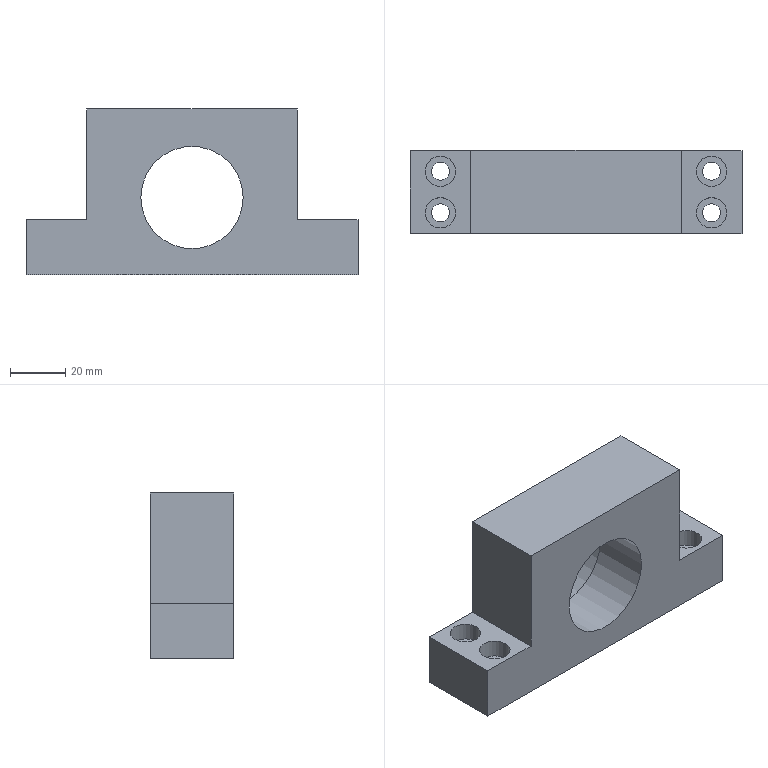Part | NX | features CBORE_HOLE 4, DATUM_CSYS 4, SKETCH 3, EXTRUDE 2, HOLE PACKAGE 1 | 1 solid | 25 faces | box 120 x 30 x 60 mm | volume 123889 mm3 | plane 15 | cylinder 10 | commonest cylinder face diameters 6.5 x4 11 x4 37 x1 42 x1
STEP:
#1=CARTESIAN_POINT('',(21.,15.,28.));
#2=VERTEX_POINT('',#1);
#3=CARTESIAN_POINT('',(0.,15.,28.));
#4=DIRECTION('',(0.,-1.,0.));
#5=DIRECTION('',(1.,0.,0.));
#6=AXIS2_PLACEMENT_3D('',#3,#4,#5);
#7=CIRCLE('',#6,21.);
#8=EDGE_CURVE('',#2,#2,#7,.T.);
#9=ORIENTED_EDGE('',*,*,#8,.F.);
#10=EDGE_LOOP('',(#9));
#11=FACE_BOUND('',#10,.T.);
#12=CARTESIAN_POINT('',(21.,6.,28.));
#13=VERTEX_POINT('',#12);
#14=CARTESIAN_POINT('',(0.,6.,28.));
#15=DIRECTION('',(0.,-1.,0.));
#16=DIRECTION('',(1.,0.,0.));
#17=AXIS2_PLACEMENT_3D('',#14,#15,#16);
#18=CIRCLE('',#17,21.);
#19=EDGE_CURVE('',#13,#13,#18,.T.);
#20=ORIENTED_EDGE('',*,*,#19,.T.);
#21=EDGE_LOOP('',(#20));
#22=FACE_BOUND('',#21,.T.);
#23=CARTESIAN_POINT('',(0.,-15.,28.));
#24=DIRECTION('',(0.,1.,0.));
#25=DIRECTION('',(0.,0.,1.));
#26=AXIS2_PLACEMENT_3D('',#23,#24,#25);
#27=CYLINDRICAL_SURFACE('',#26,21.);
#28=ADVANCED_FACE('',(#11,#22),#27,.F.);
#29=CARTESIAN_POINT('',(-60.,15.,20.));
#30=VERTEX_POINT('',#29);
#31=CARTESIAN_POINT('',(-60.,15.,0.));
#32=VERTEX_POINT('',#31);
#33=CARTESIAN_POINT('',(-60.,15.,20.));
#34=DIRECTION('',(0.,0.,-1.));
#35=VECTOR('',#34,1000.);
#36=LINE('',#33,#35);
#37=EDGE_CURVE('',#30,#32,#36,.T.);
#38=ORIENTED_EDGE('',*,*,#37,.T.);
#39=CARTESIAN_POINT('',(-60.,-15.,0.));
#40=VERTEX_POINT('',#39);
#41=CARTESIAN_POINT('',(-60.,-15.,0.));
#42=DIRECTION('',(0.,1.,0.));
#43=VECTOR('',#42,1000.);
#44=LINE('',#41,#43);
#45=EDGE_CURVE('',#40,#32,#44,.T.);
#46=ORIENTED_EDGE('',*,*,#45,.F.);
#47=CARTESIAN_POINT('',(-60.,-15.,20.));
#48=VERTEX_POINT('',#47);
#49=CARTESIAN_POINT('',(-60.,-15.,20.));
#50=DIRECTION('',(0.,0.,-1.));
#51=VECTOR('',#50,1000.);
#52=LINE('',#49,#51);
#53=EDGE_CURVE('',#48,#40,#52,.T.);
#54=ORIENTED_EDGE('',*,*,#53,.F.);
#55=CARTESIAN_POINT('',(-60.,-15.,20.));
#56=DIRECTION('',(0.,1.,0.));
#57=VECTOR('',#56,1000.);
#58=LINE('',#55,#57);
#59=EDGE_CURVE('',#48,#30,#58,.T.);
#60=ORIENTED_EDGE('',*,*,#59,.T.);
#61=EDGE_LOOP('',(#38,#46,#54,#60));
#62=FACE_BOUND('',#61,.T.);
#63=CARTESIAN_POINT('',(-60.,-15.,20.));
#64=DIRECTION('',(1.,0.,0.));
#65=DIRECTION('',(0.,0.,-1.));
#66=AXIS2_PLACEMENT_3D('',#63,#64,#65);
#67=PLANE('',#66);
#68=ADVANCED_FACE('',(#62),#67,.F.);
#69=CARTESIAN_POINT('',(52.25,7.5,0.));
#70=VERTEX_POINT('',#69);
#71=CARTESIAN_POINT('',(49.,7.5,0.));
#72=DIRECTION('',(0.,0.,1.));
#73=DIRECTION('',(1.,0.,0.));
#74=AXIS2_PLACEMENT_3D('',#71,#72,#73);
#75=CIRCLE('',#74,3.25);
#76=EDGE_CURVE('',#70,#70,#75,.T.);
#77=ORIENTED_EDGE('',*,*,#76,.T.);
#78=EDGE_LOOP('',(#77));
#79=FACE_BOUND('',#78,.T.);
#80=CARTESIAN_POINT('',(52.25,-7.5,0.));
#81=VERTEX_POINT('',#80);
#82=CARTESIAN_POINT('',(49.,-7.5,0.));
#83=DIRECTION('',(0.,0.,1.));
#84=DIRECTION('',(1.,0.,0.));
#85=AXIS2_PLACEMENT_3D('',#82,#83,#84);
#86=CIRCLE('',#85,3.25);
#87=EDGE_CURVE('',#81,#81,#86,.T.);
#88=ORIENTED_EDGE('',*,*,#87,.T.);
#89=EDGE_LOOP('',(#88));
#90=FACE_BOUND('',#89,.T.);
#91=CARTESIAN_POINT('',(-45.75,-7.5,0.));
#92=VERTEX_POINT('',#91);
#93=CARTESIAN_POINT('',(-49.,-7.5,0.));
#94=DIRECTION('',(0.,0.,1.));
#95=DIRECTION('',(1.,0.,0.));
#96=AXIS2_PLACEMENT_3D('',#93,#94,#95);
#97=CIRCLE('',#96,3.25);
#98=EDGE_CURVE('',#92,#92,#97,.T.);
#99=ORIENTED_EDGE('',*,*,#98,.T.);
#100=EDGE_LOOP('',(#99));
#101=FACE_BOUND('',#100,.T.);
#102=CARTESIAN_POINT('',(-45.75,7.5,0.));
#103=VERTEX_POINT('',#102);
#104=CARTESIAN_POINT('',(-49.,7.5,0.));
#105=DIRECTION('',(0.,0.,1.));
#106=DIRECTION('',(1.,0.,0.));
#107=AXIS2_PLACEMENT_3D('',#104,#105,#106);
#108=CIRCLE('',#107,3.25);
#109=EDGE_CURVE('',#103,#103,#108,.T.);
#110=ORIENTED_EDGE('',*,*,#109,.T.);
#111=EDGE_LOOP('',(#110));
#112=FACE_BOUND('',#111,.T.);
#113=CARTESIAN_POINT('',(60.,15.,0.));
#114=VERTEX_POINT('',#113);
#115=CARTESIAN_POINT('',(-60.,15.,0.));
#116=DIRECTION('',(1.,0.,0.));
#117=VECTOR('',#116,1000.);
#118=LINE('',#115,#117);
#119=EDGE_CURVE('',#32,#114,#118,.T.);
#120=ORIENTED_EDGE('',*,*,#119,.T.);
#121=CARTESIAN_POINT('',(60.,-15.,0.));
#122=VERTEX_POINT('',#121);
#123=CARTESIAN_POINT('',(60.,-15.,0.));
#124=DIRECTION('',(0.,1.,0.));
#125=VECTOR('',#124,1000.);
#126=LINE('',#123,#125);
#127=EDGE_CURVE('',#122,#114,#126,.T.);
#128=ORIENTED_EDGE('',*,*,#127,.F.);
#129=CARTESIAN_POINT('',(-60.,-15.,0.));
#130=DIRECTION('',(1.,0.,0.));
#131=VECTOR('',#130,1000.);
#132=LINE('',#129,#131);
#133=EDGE_CURVE('',#40,#122,#132,.T.);
#134=ORIENTED_EDGE('',*,*,#133,.F.);
#135=ORIENTED_EDGE('',*,*,#45,.T.);
#136=EDGE_LOOP('',(#120,#128,#134,#135));
#137=FACE_BOUND('',#136,.T.);
#138=CARTESIAN_POINT('',(-60.,-15.,0.));
#139=DIRECTION('',(0.,0.,1.));
#140=DIRECTION('',(1.,0.,0.));
#141=AXIS2_PLACEMENT_3D('',#138,#139,#140);
#142=PLANE('',#141);
#143=ADVANCED_FACE('',(#79,#90,#101,#112,#137),#142,.F.);
#144=CARTESIAN_POINT('',(60.,15.,20.));
#145=VERTEX_POINT('',#144);
#146=CARTESIAN_POINT('',(60.,15.,0.));
#147=DIRECTION('',(0.,0.,1.));
#148=VECTOR('',#147,1000.);
#149=LINE('',#146,#148);
#150=EDGE_CURVE('',#114,#145,#149,.T.);
#151=ORIENTED_EDGE('',*,*,#150,.T.);
#152=CARTESIAN_POINT('',(60.,-15.,20.));
#153=VERTEX_POINT('',#152);
#154=CARTESIAN_POINT('',(60.,-15.,20.));
#155=DIRECTION('',(0.,1.,0.));
#156=VECTOR('',#155,1000.);
#157=LINE('',#154,#156);
#158=EDGE_CURVE('',#153,#145,#157,.T.);
#159=ORIENTED_EDGE('',*,*,#158,.F.);
#160=CARTESIAN_POINT('',(60.,-15.,0.));
#161=DIRECTION('',(0.,0.,1.));
#162=VECTOR('',#161,1000.);
#163=LINE('',#160,#162);
#164=EDGE_CURVE('',#122,#153,#163,.T.);
#165=ORIENTED_EDGE('',*,*,#164,.F.);
#166=ORIENTED_EDGE('',*,*,#127,.T.);
#167=EDGE_LOOP('',(#151,#159,#165,#166));
#168=FACE_BOUND('',#167,.T.);
#169=CARTESIAN_POINT('',(60.,-15.,0.));
#170=DIRECTION('',(-1.,0.,0.));
#171=DIRECTION('',(0.,0.,1.));
#172=AXIS2_PLACEMENT_3D('',#169,#170,#171);
#173=PLANE('',#172);
#174=ADVANCED_FACE('',(#168),#173,.F.);
#175=CARTESIAN_POINT('',(43.5,7.5,20.));
#176=VERTEX_POINT('',#175);
#177=CARTESIAN_POINT('',(49.,7.5,20.));
#178=DIRECTION('',(0.,0.,-1.));
#179=DIRECTION('',(-1.,0.,0.));
#180=AXIS2_PLACEMENT_3D('',#177,#178,#179);
#181=CIRCLE('',#180,5.5);
#182=EDGE_CURVE('',#176,#176,#181,.T.);
#183=ORIENTED_EDGE('',*,*,#182,.T.);
#184=EDGE_LOOP('',(#183));
#185=FACE_BOUND('',#184,.T.);
#186=CARTESIAN_POINT('',(43.5,-7.5,20.));
#187=VERTEX_POINT('',#186);
#188=CARTESIAN_POINT('',(49.,-7.5,20.));
#189=DIRECTION('',(0.,0.,-1.));
#190=DIRECTION('',(-1.,0.,0.));
#191=AXIS2_PLACEMENT_3D('',#188,#189,#190);
#192=CIRCLE('',#191,5.5);
#193=EDGE_CURVE('',#187,#187,#192,.T.);
#194=ORIENTED_EDGE('',*,*,#193,.T.);
#195=EDGE_LOOP('',(#194));
#196=FACE_BOUND('',#195,.T.);
#197=CARTESIAN_POINT('',(38.,15.,20.));
#198=VERTEX_POINT('',#197);
#199=CARTESIAN_POINT('',(60.,15.,20.));
#200=DIRECTION('',(-1.,0.,0.));
#201=VECTOR('',#200,1000.);
#202=LINE('',#199,#201);
#203=EDGE_CURVE('',#145,#198,#202,.T.);
#204=ORIENTED_EDGE('',*,*,#203,.T.);
#205=CARTESIAN_POINT('',(38.,-15.,20.));
#206=VERTEX_POINT('',#205);
#207=CARTESIAN_POINT('',(38.,-15.,20.));
#208=DIRECTION('',(0.,1.,0.));
#209=VECTOR('',#208,1000.);
#210=LINE('',#207,#209);
#211=EDGE_CURVE('',#206,#198,#210,.T.);
#212=ORIENTED_EDGE('',*,*,#211,.F.);
#213=CARTESIAN_POINT('',(60.,-15.,20.));
#214=DIRECTION('',(-1.,0.,0.));
#215=VECTOR('',#214,1000.);
#216=LINE('',#213,#215);
#217=EDGE_CURVE('',#153,#206,#216,.T.);
#218=ORIENTED_EDGE('',*,*,#217,.F.);
#219=ORIENTED_EDGE('',*,*,#158,.T.);
#220=EDGE_LOOP('',(#204,#212,#218,#219));
#221=FACE_BOUND('',#220,.T.);
#222=CARTESIAN_POINT('',(60.,-15.,20.));
#223=DIRECTION('',(0.,0.,-1.));
#224=DIRECTION('',(-1.,0.,0.));
#225=AXIS2_PLACEMENT_3D('',#222,#223,#224);
#226=PLANE('',#225);
#227=ADVANCED_FACE('',(#185,#196,#221),#226,.F.);
#228=CARTESIAN_POINT('',(38.,15.,60.));
#229=VERTEX_POINT('',#228);
#230=CARTESIAN_POINT('',(38.,15.,20.));
#231=DIRECTION('',(0.,0.,1.));
#232=VECTOR('',#231,1000.);
#233=LINE('',#230,#232);
#234=EDGE_CURVE('',#198,#229,#233,.T.);
#235=ORIENTED_EDGE('',*,*,#234,.T.);
#236=CARTESIAN_POINT('',(38.,-15.,60.));
#237=VERTEX_POINT('',#236);
#238=CARTESIAN_POINT('',(38.,-15.,60.));
#239=DIRECTION('',(0.,1.,0.));
#240=VECTOR('',#239,1000.);
#241=LINE('',#238,#240);
#242=EDGE_CURVE('',#237,#229,#241,.T.);
#243=ORIENTED_EDGE('',*,*,#242,.F.);
#244=CARTESIAN_POINT('',(38.,-15.,20.));
#245=DIRECTION('',(0.,0.,1.));
#246=VECTOR('',#245,1000.);
#247=LINE('',#244,#246);
#248=EDGE_CURVE('',#206,#237,#247,.T.);
#249=ORIENTED_EDGE('',*,*,#248,.F.);
#250=ORIENTED_EDGE('',*,*,#211,.T.);
#251=EDGE_LOOP('',(#235,#243,#249,#250));
#252=FACE_BOUND('',#251,.T.);
#253=CARTESIAN_POINT('',(38.,-15.,20.));
#254=DIRECTION('',(-1.,0.,0.));
#255=DIRECTION('',(0.,0.,1.));
#256=AXIS2_PLACEMENT_3D('',#253,#254,#255);
#257=PLANE('',#256);
#258=ADVANCED_FACE('',(#252),#257,.F.);
#259=CARTESIAN_POINT('',(-38.,15.,60.));
#260=VERTEX_POINT('',#259);
#261=CARTESIAN_POINT('',(38.,15.,60.));
#262=DIRECTION('',(-1.,0.,0.));
#263=VECTOR('',#262,1000.);
#264=LINE('',#261,#263);
#265=EDGE_CURVE('',#229,#260,#264,.T.);
#266=ORIENTED_EDGE('',*,*,#265,.T.);
#267=CARTESIAN_POINT('',(-38.,-15.,60.));
#268=VERTEX_POINT('',#267);
#269=CARTESIAN_POINT('',(-38.,-15.,60.));
#270=DIRECTION('',(0.,1.,0.));
#271=VECTOR('',#270,1000.);
#272=LINE('',#269,#271);
#273=EDGE_CURVE('',#268,#260,#272,.T.);
#274=ORIENTED_EDGE('',*,*,#273,.F.);
#275=CARTESIAN_POINT('',(38.,-15.,60.));
#276=DIRECTION('',(-1.,0.,0.));
#277=VECTOR('',#276,1000.);
#278=LINE('',#275,#277);
#279=EDGE_CURVE('',#237,#268,#278,.T.);
#280=ORIENTED_EDGE('',*,*,#279,.F.);
#281=ORIENTED_EDGE('',*,*,#242,.T.);
#282=EDGE_LOOP('',(#266,#274,#280,#281));
#283=FACE_BOUND('',#282,.T.);
#284=CARTESIAN_POINT('',(38.,-15.,60.));
#285=DIRECTION('',(0.,0.,-1.));
#286=DIRECTION('',(-1.,0.,0.));
#287=AXIS2_PLACEMENT_3D('',#284,#285,#286);
#288=PLANE('',#287);
#289=ADVANCED_FACE('',(#283),#288,.F.);
#290=CARTESIAN_POINT('',(-38.,15.,20.));
#291=VERTEX_POINT('',#290);
#292=CARTESIAN_POINT('',(-38.,15.,60.));
#293=DIRECTION('',(0.,0.,-1.));
#294=VECTOR('',#293,1000.);
#295=LINE('',#292,#294);
#296=EDGE_CURVE('',#260,#291,#295,.T.);
#297=ORIENTED_EDGE('',*,*,#296,.T.);
#298=CARTESIAN_POINT('',(-38.,-15.,20.));
#299=VERTEX_POINT('',#298);
#300=CARTESIAN_POINT('',(-38.,-15.,20.));
#301=DIRECTION('',(0.,1.,0.));
#302=VECTOR('',#301,1000.);
#303=LINE('',#300,#302);
#304=EDGE_CURVE('',#299,#291,#303,.T.);
#305=ORIENTED_EDGE('',*,*,#304,.F.);
#306=CARTESIAN_POINT('',(-38.,-15.,60.));
#307=DIRECTION('',(0.,0.,-1.));
#308=VECTOR('',#307,1000.);
#309=LINE('',#306,#308);
#310=EDGE_CURVE('',#268,#299,#309,.T.);
#311=ORIENTED_EDGE('',*,*,#310,.F.);
#312=ORIENTED_EDGE('',*,*,#273,.T.);
#313=EDGE_LOOP('',(#297,#305,#311,#312));
#314=FACE_BOUND('',#313,.T.);
#315=CARTESIAN_POINT('',(-38.,-15.,60.));
#316=DIRECTION('',(1.,0.,0.));
#317=DIRECTION('',(0.,0.,-1.));
#318=AXIS2_PLACEMENT_3D('',#315,#316,#317);
#319=PLANE('',#318);
#320=ADVANCED_FACE('',(#314),#319,.F.);
#321=CARTESIAN_POINT('',(-54.5,-7.5,20.));
#322=VERTEX_POINT('',#321);
#323=CARTESIAN_POINT('',(-49.,-7.5,20.));
#324=DIRECTION('',(0.,0.,-1.));
#325=DIRECTION('',(-1.,0.,0.));
#326=AXIS2_PLACEMENT_3D('',#323,#324,#325);
#327=CIRCLE('',#326,5.5);
#328=EDGE_CURVE('',#322,#322,#327,.T.);
#329=ORIENTED_EDGE('',*,*,#328,.T.);
#330=EDGE_LOOP('',(#329));
#331=FACE_BOUND('',#330,.T.);
#332=CARTESIAN_POINT('',(-54.5,7.5,20.));
#333=VERTEX_POINT('',#332);
#334=CARTESIAN_POINT('',(-49.,7.5,20.));
#335=DIRECTION('',(0.,0.,-1.));
#336=DIRECTION('',(-1.,0.,0.));
#337=AXIS2_PLACEMENT_3D('',#334,#335,#336);
#338=CIRCLE('',#337,5.5);
#339=EDGE_CURVE('',#333,#333,#338,.T.);
#340=ORIENTED_EDGE('',*,*,#339,.T.);
#341=EDGE_LOOP('',(#340));
#342=FACE_BOUND('',#341,.T.);
#343=CARTESIAN_POINT('',(-38.,15.,20.));
#344=DIRECTION('',(-1.,0.,0.));
#345=VECTOR('',#344,1000.);
#346=LINE('',#343,#345);
#347=EDGE_CURVE('',#291,#30,#346,.T.);
#348=ORIENTED_EDGE('',*,*,#347,.T.);
#349=ORIENTED_EDGE('',*,*,#59,.F.);
#350=CARTESIAN_POINT('',(-38.,-15.,20.));
#351=DIRECTION('',(-1.,0.,0.));
#352=VECTOR('',#351,1000.);
#353=LINE('',#350,#352);
#354=EDGE_CURVE('',#299,#48,#353,.T.);
#355=ORIENTED_EDGE('',*,*,#354,.F.);
#356=ORIENTED_EDGE('',*,*,#304,.T.);
#357=EDGE_LOOP('',(#348,#349,#355,#356));
#358=FACE_BOUND('',#357,.T.);
#359=CARTESIAN_POINT('',(-38.,-15.,20.));
#360=DIRECTION('',(0.,0.,-1.));
#361=DIRECTION('',(-1.,0.,0.));
#362=AXIS2_PLACEMENT_3D('',#359,#360,#361);
#363=PLANE('',#362);
#364=ADVANCED_FACE('',(#331,#342,#358),#363,.F.);
#365=ORIENTED_EDGE('',*,*,#53,.T.);
#366=ORIENTED_EDGE('',*,*,#133,.T.);
#367=ORIENTED_EDGE('',*,*,#164,.T.);
#368=ORIENTED_EDGE('',*,*,#217,.T.);
#369=ORIENTED_EDGE('',*,*,#248,.T.);
#370=ORIENTED_EDGE('',*,*,#279,.T.);
#371=ORIENTED_EDGE('',*,*,#310,.T.);
#372=ORIENTED_EDGE('',*,*,#354,.T.);
#373=EDGE_LOOP('',(#365,#366,#367,#368,#369,#370,#371,#372));
#374=FACE_BOUND('',#373,.T.);
#375=CARTESIAN_POINT('',(18.5,-15.,28.));
#376=VERTEX_POINT('',#375);
#377=CARTESIAN_POINT('',(0.,-15.,28.));
#378=DIRECTION('',(0.,-1.,0.));
#379=DIRECTION('',(1.,0.,0.));
#380=AXIS2_PLACEMENT_3D('',#377,#378,#379);
#381=CIRCLE('',#380,18.5);
#382=EDGE_CURVE('',#376,#376,#381,.T.);
#383=ORIENTED_EDGE('',*,*,#382,.F.);
#384=EDGE_LOOP('',(#383));
#385=FACE_BOUND('',#384,.T.);
#386=CARTESIAN_POINT('',(0.,-15.,28.));
#387=DIRECTION('',(0.,-1.,0.));
#388=DIRECTION('',(0.,0.,-1.));
#389=AXIS2_PLACEMENT_3D('',#386,#387,#388);
#390=PLANE('',#389);
#391=ADVANCED_FACE('',(#374,#385),#390,.T.);
#392=ORIENTED_EDGE('',*,*,#37,.F.);
#393=ORIENTED_EDGE('',*,*,#347,.F.);
#394=ORIENTED_EDGE('',*,*,#296,.F.);
#395=ORIENTED_EDGE('',*,*,#265,.F.);
#396=ORIENTED_EDGE('',*,*,#234,.F.);
#397=ORIENTED_EDGE('',*,*,#203,.F.);
#398=ORIENTED_EDGE('',*,*,#150,.F.);
#399=ORIENTED_EDGE('',*,*,#119,.F.);
#400=EDGE_LOOP('',(#392,#393,#394,#395,#396,#397,#398,#399));
#401=FACE_BOUND('',#400,.T.);
#402=ORIENTED_EDGE('',*,*,#8,.T.);
#403=EDGE_LOOP('',(#402));
#404=FACE_BOUND('',#403,.T.);
#405=CARTESIAN_POINT('',(0.,15.,28.));
#406=DIRECTION('',(0.,-1.,0.));
#407=DIRECTION('',(0.,0.,-1.));
#408=AXIS2_PLACEMENT_3D('',#405,#406,#407);
#409=PLANE('',#408);
#410=ADVANCED_FACE('',(#401,#404),#409,.F.);
#411=CARTESIAN_POINT('',(18.5,6.,28.));
#412=VERTEX_POINT('',#411);
#413=CARTESIAN_POINT('',(0.,6.,28.));
#414=DIRECTION('',(0.,-1.,0.));
#415=DIRECTION('',(1.,0.,0.));
#416=AXIS2_PLACEMENT_3D('',#413,#414,#415);
#417=CIRCLE('',#416,18.5);
#418=EDGE_CURVE('',#412,#412,#417,.T.);
#419=ORIENTED_EDGE('',*,*,#418,.F.);
#420=EDGE_LOOP('',(#419));
#421=FACE_BOUND('',#420,.T.);
#422=ORIENTED_EDGE('',*,*,#382,.T.);
#423=EDGE_LOOP('',(#422));
#424=FACE_BOUND('',#423,.T.);
#425=CARTESIAN_POINT('',(0.,6.,28.));
#426=DIRECTION('',(0.,-1.,0.));
#427=DIRECTION('',(0.,0.,-1.));
#428=AXIS2_PLACEMENT_3D('',#425,#426,#427);
#429=CYLINDRICAL_SURFACE('',#428,18.5);
#430=ADVANCED_FACE('',(#421,#424),#429,.F.);
#431=ORIENTED_EDGE('',*,*,#19,.F.);
#432=EDGE_LOOP('',(#431));
#433=FACE_BOUND('',#432,.T.);
#434=ORIENTED_EDGE('',*,*,#418,.T.);
#435=EDGE_LOOP('',(#434));
#436=FACE_BOUND('',#435,.T.);
#437=CARTESIAN_POINT('',(0.,6.,28.));
#438=DIRECTION('',(0.,-1.,0.));
#439=DIRECTION('',(0.,0.,-1.));
#440=AXIS2_PLACEMENT_3D('',#437,#438,#439);
#441=PLANE('',#440);
#442=ADVANCED_FACE('',(#433,#436),#441,.F.);
#443=CARTESIAN_POINT('',(-52.25,7.5,13.5));
#444=VERTEX_POINT('',#443);
#445=CARTESIAN_POINT('',(-49.,7.5,13.5));
#446=DIRECTION('',(0.,0.,-1.));
#447=DIRECTION('',(-1.,0.,0.));
#448=AXIS2_PLACEMENT_3D('',#445,#446,#447);
#449=CIRCLE('',#448,3.25);
#450=EDGE_CURVE('',#444,#444,#449,.F.);
#451=ORIENTED_EDGE('',*,*,#450,.T.);
#452=EDGE_LOOP('',(#451));
#453=FACE_BOUND('',#452,.T.);
#454=ORIENTED_EDGE('',*,*,#109,.F.);
#455=EDGE_LOOP('',(#454));
#456=FACE_BOUND('',#455,.T.);
#457=CARTESIAN_POINT('',(-49.,7.5,-27.096));
#458=DIRECTION('',(0.,0.,-1.));
#459=DIRECTION('',(-1.,0.,0.));
#460=AXIS2_PLACEMENT_3D('',#457,#458,#459);
#461=CYLINDRICAL_SURFACE('',#460,3.25);
#462=ADVANCED_FACE('',(#453,#456),#461,.F.);
#463=ORIENTED_EDGE('',*,*,#450,.F.);
#464=EDGE_LOOP('',(#463));
#465=FACE_BOUND('',#464,.T.);
#466=CARTESIAN_POINT('',(-54.5,7.5,13.5));
#467=VERTEX_POINT('',#466);
#468=CARTESIAN_POINT('',(-49.,7.5,13.5));
#469=DIRECTION('',(0.,0.,-1.));
#470=DIRECTION('',(-1.,0.,0.));
#471=AXIS2_PLACEMENT_3D('',#468,#469,#470);
#472=CIRCLE('',#471,5.5);
#473=EDGE_CURVE('',#467,#467,#472,.F.);
#474=ORIENTED_EDGE('',*,*,#473,.T.);
#475=EDGE_LOOP('',(#474));
#476=FACE_BOUND('',#475,.T.);
#477=CARTESIAN_POINT('',(-49.,7.5,13.5));
#478=DIRECTION('',(0.,0.,-1.));
#479=DIRECTION('',(-1.,0.,0.));
#480=AXIS2_PLACEMENT_3D('',#477,#478,#479);
#481=PLANE('',#480);
#482=ADVANCED_FACE('',(#465,#476),#481,.F.);
#483=ORIENTED_EDGE('',*,*,#473,.F.);
#484=EDGE_LOOP('',(#483));
#485=FACE_BOUND('',#484,.T.);
#486=ORIENTED_EDGE('',*,*,#339,.F.);
#487=EDGE_LOOP('',(#486));
#488=FACE_BOUND('',#487,.T.);
#489=CARTESIAN_POINT('',(-49.,7.5,20.));
#490=DIRECTION('',(0.,0.,-1.));
#491=DIRECTION('',(-1.,0.,0.));
#492=AXIS2_PLACEMENT_3D('',#489,#490,#491);
#493=CYLINDRICAL_SURFACE('',#492,5.5);
#494=ADVANCED_FACE('',(#485,#488),#493,.F.);
#495=CARTESIAN_POINT('',(-52.25,-7.5,13.5));
#496=VERTEX_POINT('',#495);
#497=CARTESIAN_POINT('',(-49.,-7.5,13.5));
#498=DIRECTION('',(0.,0.,-1.));
#499=DIRECTION('',(-1.,0.,0.));
#500=AXIS2_PLACEMENT_3D('',#497,#498,#499);
#501=CIRCLE('',#500,3.25);
#502=EDGE_CURVE('',#496,#496,#501,.F.);
#503=ORIENTED_EDGE('',*,*,#502,.T.);
#504=EDGE_LOOP('',(#503));
#505=FACE_BOUND('',#504,.T.);
#506=ORIENTED_EDGE('',*,*,#98,.F.);
#507=EDGE_LOOP('',(#506));
#508=FACE_BOUND('',#507,.T.);
#509=CARTESIAN_POINT('',(-49.,-7.5,-27.096));
#510=DIRECTION('',(0.,0.,-1.));
#511=DIRECTION('',(-1.,0.,0.));
#512=AXIS2_PLACEMENT_3D('',#509,#510,#511);
#513=CYLINDRICAL_SURFACE('',#512,3.25);
#514=ADVANCED_FACE('',(#505,#508),#513,.F.);
#515=ORIENTED_EDGE('',*,*,#502,.F.);
#516=EDGE_LOOP('',(#515));
#517=FACE_BOUND('',#516,.T.);
#518=CARTESIAN_POINT('',(-54.5,-7.5,13.5));
#519=VERTEX_POINT('',#518);
#520=CARTESIAN_POINT('',(-49.,-7.5,13.5));
#521=DIRECTION('',(0.,0.,-1.));
#522=DIRECTION('',(-1.,0.,0.));
#523=AXIS2_PLACEMENT_3D('',#520,#521,#522);
#524=CIRCLE('',#523,5.5);
#525=EDGE_CURVE('',#519,#519,#524,.F.);
#526=ORIENTED_EDGE('',*,*,#525,.T.);
#527=EDGE_LOOP('',(#526));
#528=FACE_BOUND('',#527,.T.);
#529=CARTESIAN_POINT('',(-49.,-7.5,13.5));
#530=DIRECTION('',(0.,0.,-1.));
#531=DIRECTION('',(-1.,0.,0.));
#532=AXIS2_PLACEMENT_3D('',#529,#530,#531);
#533=PLANE('',#532);
#534=ADVANCED_FACE('',(#517,#528),#533,.F.);
#535=ORIENTED_EDGE('',*,*,#525,.F.);
#536=EDGE_LOOP('',(#535));
#537=FACE_BOUND('',#536,.T.);
#538=ORIENTED_EDGE('',*,*,#328,.F.);
#539=EDGE_LOOP('',(#538));
#540=FACE_BOUND('',#539,.T.);
#541=CARTESIAN_POINT('',(-49.,-7.5,20.));
#542=DIRECTION('',(0.,0.,-1.));
#543=DIRECTION('',(-1.,0.,0.));
#544=AXIS2_PLACEMENT_3D('',#541,#542,#543);
#545=CYLINDRICAL_SURFACE('',#544,5.5);
#546=ADVANCED_FACE('',(#537,#540),#545,.F.);
#547=CARTESIAN_POINT('',(45.75,-7.5,13.5));
#548=VERTEX_POINT('',#547);
#549=CARTESIAN_POINT('',(49.,-7.5,13.5));
#550=DIRECTION('',(0.,0.,-1.));
#551=DIRECTION('',(-1.,0.,0.));
#552=AXIS2_PLACEMENT_3D('',#549,#550,#551);
#553=CIRCLE('',#552,3.25);
#554=EDGE_CURVE('',#548,#548,#553,.F.);
#555=ORIENTED_EDGE('',*,*,#554,.T.);
#556=EDGE_LOOP('',(#555));
#557=FACE_BOUND('',#556,.T.);
#558=ORIENTED_EDGE('',*,*,#87,.F.);
#559=EDGE_LOOP('',(#558));
#560=FACE_BOUND('',#559,.T.);
#561=CARTESIAN_POINT('',(49.,-7.5,-27.096));
#562=DIRECTION('',(0.,0.,-1.));
#563=DIRECTION('',(-1.,0.,0.));
#564=AXIS2_PLACEMENT_3D('',#561,#562,#563);
#565=CYLINDRICAL_SURFACE('',#564,3.25);
#566=ADVANCED_FACE('',(#557,#560),#565,.F.);
#567=ORIENTED_EDGE('',*,*,#554,.F.);
#568=EDGE_LOOP('',(#567));
#569=FACE_BOUND('',#568,.T.);
#570=CARTESIAN_POINT('',(43.5,-7.5,13.5));
#571=VERTEX_POINT('',#570);
#572=CARTESIAN_POINT('',(49.,-7.5,13.5));
#573=DIRECTION('',(0.,0.,-1.));
#574=DIRECTION('',(-1.,0.,0.));
#575=AXIS2_PLACEMENT_3D('',#572,#573,#574);
#576=CIRCLE('',#575,5.5);
#577=EDGE_CURVE('',#571,#571,#576,.F.);
#578=ORIENTED_EDGE('',*,*,#577,.T.);
#579=EDGE_LOOP('',(#578));
#580=FACE_BOUND('',#579,.T.);
#581=CARTESIAN_POINT('',(49.,-7.5,13.5));
#582=DIRECTION('',(0.,0.,-1.));
#583=DIRECTION('',(-1.,0.,0.));
#584=AXIS2_PLACEMENT_3D('',#581,#582,#583);
#585=PLANE('',#584);
#586=ADVANCED_FACE('',(#569,#580),#585,.F.);
#587=ORIENTED_EDGE('',*,*,#577,.F.);
#588=EDGE_LOOP('',(#587));
#589=FACE_BOUND('',#588,.T.);
#590=ORIENTED_EDGE('',*,*,#193,.F.);
#591=EDGE_LOOP('',(#590));
#592=FACE_BOUND('',#591,.T.);
#593=CARTESIAN_POINT('',(49.,-7.5,20.));
#594=DIRECTION('',(0.,0.,-1.));
#595=DIRECTION('',(-1.,0.,0.));
#596=AXIS2_PLACEMENT_3D('',#593,#594,#595);
#597=CYLINDRICAL_SURFACE('',#596,5.5);
#598=ADVANCED_FACE('',(#589,#592),#597,.F.);
#599=CARTESIAN_POINT('',(45.75,7.5,13.5));
#600=VERTEX_POINT('',#599);
#601=CARTESIAN_POINT('',(49.,7.5,13.5));
#602=DIRECTION('',(0.,0.,-1.));
#603=DIRECTION('',(-1.,0.,0.));
#604=AXIS2_PLACEMENT_3D('',#601,#602,#603);
#605=CIRCLE('',#604,3.25);
#606=EDGE_CURVE('',#600,#600,#605,.F.);
#607=ORIENTED_EDGE('',*,*,#606,.T.);
#608=EDGE_LOOP('',(#607));
#609=FACE_BOUND('',#608,.T.);
#610=ORIENTED_EDGE('',*,*,#76,.F.);
#611=EDGE_LOOP('',(#610));
#612=FACE_BOUND('',#611,.T.);
#613=CARTESIAN_POINT('',(49.,7.5,-27.096));
#614=DIRECTION('',(0.,0.,-1.));
#615=DIRECTION('',(-1.,0.,0.));
#616=AXIS2_PLACEMENT_3D('',#613,#614,#615);
#617=CYLINDRICAL_SURFACE('',#616,3.25);
#618=ADVANCED_FACE('',(#609,#612),#617,.F.);
#619=ORIENTED_EDGE('',*,*,#606,.F.);
#620=EDGE_LOOP('',(#619));
#621=FACE_BOUND('',#620,.T.);
#622=CARTESIAN_POINT('',(43.5,7.5,13.5));
#623=VERTEX_POINT('',#622);
#624=CARTESIAN_POINT('',(49.,7.5,13.5));
#625=DIRECTION('',(0.,0.,-1.));
#626=DIRECTION('',(-1.,0.,0.));
#627=AXIS2_PLACEMENT_3D('',#624,#625,#626);
#628=CIRCLE('',#627,5.5);
#629=EDGE_CURVE('',#623,#623,#628,.F.);
#630=ORIENTED_EDGE('',*,*,#629,.T.);
#631=EDGE_LOOP('',(#630));
#632=FACE_BOUND('',#631,.T.);
#633=CARTESIAN_POINT('',(49.,7.5,13.5));
#634=DIRECTION('',(0.,0.,-1.));
#635=DIRECTION('',(-1.,0.,0.));
#636=AXIS2_PLACEMENT_3D('',#633,#634,#635);
#637=PLANE('',#636);
#638=ADVANCED_FACE('',(#621,#632),#637,.F.);
#639=ORIENTED_EDGE('',*,*,#629,.F.);
#640=EDGE_LOOP('',(#639));
#641=FACE_BOUND('',#640,.T.);
#642=ORIENTED_EDGE('',*,*,#182,.F.);
#643=EDGE_LOOP('',(#642));
#644=FACE_BOUND('',#643,.T.);
#645=CARTESIAN_POINT('',(49.,7.5,20.));
#646=DIRECTION('',(0.,0.,-1.));
#647=DIRECTION('',(-1.,0.,0.));
#648=AXIS2_PLACEMENT_3D('',#645,#646,#647);
#649=CYLINDRICAL_SURFACE('',#648,5.5);
#650=ADVANCED_FACE('',(#641,#644),#649,.F.);
#651=CLOSED_SHELL('',(#28,#68,#143,#174,#227,#258,#289,#320,#364,#391,#410,#430,#442,#462,#482,#494,#514,#534,#546,#566,#586,#598,#618,#638,#650));
#652=MANIFOLD_SOLID_BREP('',#651);
#653=(LENGTH_UNIT()NAMED_UNIT(*)SI_UNIT(.MILLI.,.METRE.));
#654=UNCERTAINTY_MEASURE_WITH_UNIT(LENGTH_MEASURE(0.00001),#653,'','');
#655=(NAMED_UNIT(*)PLANE_ANGLE_UNIT()SI_UNIT($,.RADIAN.));
#656=(NAMED_UNIT(*)SI_UNIT($,.STERADIAN.)SOLID_ANGLE_UNIT());
#657=(GEOMETRIC_REPRESENTATION_CONTEXT(3)GLOBAL_UNCERTAINTY_ASSIGNED_CONTEXT((#654))GLOBAL_UNIT_ASSIGNED_CONTEXT((#653,#655,#656))REPRESENTATION_CONTEXT('',''));
#658=ADVANCED_BREP_SHAPE_REPRESENTATION('',(#652),#657);